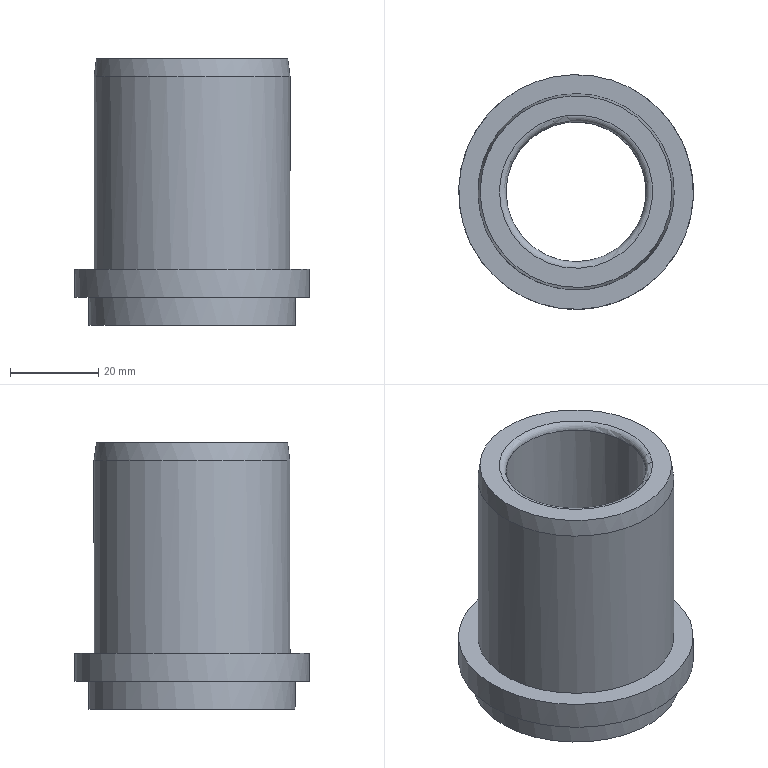Part | STEP file | 1_id1126_x_t | 1 solid | 11 faces | box 53.213 x 53.213 x 60.325 mm | volume 50805 mm3 | plane 4 | cylinder 4 | torus 2 | cone 1 | commonest cylinder face diameters 31.75 x1 44.45 x1 46.812 x1 53.213 x1
STEP:
#1=CARTESIAN_POINT('',(0.,0.,0.));
#2=DIRECTION('',(0.,0.,1.));
#3=DIRECTION('',(1.,0.,0.));
#4=AXIS2_PLACEMENT_3D('',#1,#2,#3);
#5=CARTESIAN_POINT('',(81.739,358.363,137.735));
#6=VERTEX_POINT('',#5);
#7=CARTESIAN_POINT('',(62.925,347.5,137.735));
#8=DIRECTION('',(0.,0.,1.));
#9=DIRECTION('',(0.866,0.5,0.));
#10=AXIS2_PLACEMENT_3D('',#7,#8,#9);
#11=CIRCLE('',#10,21.725);
#12=CARTESIAN_POINT('',(45.604,337.5,137.735));
#13=DIRECTION('',(0.,0.,1.));
#14=DIRECTION('',(-0.866,-0.5,0.));
#15=AXIS2_PLACEMENT_3D('',#12,#13,#14);
#16=PLANE('',#15);
#17=CARTESIAN_POINT('',(-20.,0.));
#18=DIRECTION('',(-1.,0.));
#19=AXIS2_PLACEMENT_2D('',#17,#18);
#20=CIRCLE('',#19,21.725);
#21=(GEOMETRIC_REPRESENTATION_CONTEXT(2)PARAMETRIC_REPRESENTATION_CONTEXT()REPRESENTATION_CONTEXT('',''));
#22=DEFINITIONAL_REPRESENTATION('',(#20),#21);
#23=PCURVE('',#16,#22);
#24=CARTESIAN_POINT('',(62.925,347.5,135.735));
#25=DIRECTION('',(0.,0.,-1.));
#26=DIRECTION('',(0.866,0.5,0.));
#27=AXIS2_PLACEMENT_3D('',#24,#25,#26);
#28=CONICAL_SURFACE('',#27,21.975,0.1244);
#29=CARTESIAN_POINT('',(6.283,-2.));
#30=DIRECTION('',(-1.,0.));
#31=VECTOR('',#30,1.);
#32=LINE('',#29,#31);
#33=(GEOMETRIC_REPRESENTATION_CONTEXT(2)PARAMETRIC_REPRESENTATION_CONTEXT()REPRESENTATION_CONTEXT('',''));
#34=DEFINITIONAL_REPRESENTATION('',(#32),#33);
#35=PCURVE('',#28,#34);
#36=SURFACE_CURVE('',#11,(#23,#35),.PCURVE_S1.);
#37=EDGE_CURVE('',#6,#6,#36,.T.);
#38=ORIENTED_EDGE('',*,*,#37,.T.);
#39=EDGE_LOOP('',(#38));
#40=FACE_BOUND('',#39,.T.);
#41=CARTESIAN_POINT('',(77.972,356.188,137.735));
#42=VERTEX_POINT('',#41);
#43=CARTESIAN_POINT('',(54.237,362.547,137.735));
#44=VERTEX_POINT('',#43);
#45=CARTESIAN_POINT('',(62.925,347.5,137.735));
#46=DIRECTION('',(0.,0.,-1.));
#47=DIRECTION('',(0.866,0.5,0.));
#48=AXIS2_PLACEMENT_3D('',#45,#46,#47);
#49=CIRCLE('',#48,17.375);
#50=CARTESIAN_POINT('',(-37.375,0.));
#51=CARTESIAN_POINT('',(-37.375,30.094));
#52=CARTESIAN_POINT('',(-11.312,15.047));
#53=CARTESIAN_POINT('',(14.75,0.));
#54=CARTESIAN_POINT('',(-11.312,-15.047));
#55=CARTESIAN_POINT('',(-37.375,-30.094));
#56=CARTESIAN_POINT('',(-37.375,0.));
#57=(BOUNDED_CURVE()B_SPLINE_CURVE(2,(#50,#51,#52,#53,#54,#55,#56),.UNSPECIFIED.,.T.,.F.)B_SPLINE_CURVE_WITH_KNOTS((1,2,2,2,2,1),(-2.094,0.,2.094,4.189,6.283,8.378),.UNSPECIFIED.)CURVE()GEOMETRIC_REPRESENTATION_ITEM()RATIONAL_B_SPLINE_CURVE((1.,0.5,1.,0.5,1.,0.5,1.))REPRESENTATION_ITEM(''));
#58=(GEOMETRIC_REPRESENTATION_CONTEXT(2)PARAMETRIC_REPRESENTATION_CONTEXT()REPRESENTATION_CONTEXT('',''));
#59=DEFINITIONAL_REPRESENTATION('',(#57),#58);
#60=PCURVE('',#16,#59);
#61=CARTESIAN_POINT('',(62.925,347.5,136.235));
#62=DIRECTION('',(0.,0.,1.));
#63=DIRECTION('',(-0.866,-0.5,0.));
#64=AXIS2_PLACEMENT_3D('',#61,#62,#63);
#65=TOROIDAL_SURFACE('',#64,17.375,1.5);
#66=CARTESIAN_POINT('',(9.425,7.854));
#67=DIRECTION('',(-1.,0.));
#68=VECTOR('',#67,1.);
#69=LINE('',#66,#68);
#70=(GEOMETRIC_REPRESENTATION_CONTEXT(2)PARAMETRIC_REPRESENTATION_CONTEXT()REPRESENTATION_CONTEXT('',''));
#71=DEFINITIONAL_REPRESENTATION('',(#69),#70);
#72=PCURVE('',#65,#71);
#73=SURFACE_CURVE('',#49,(#60,#72),.PCURVE_S1.);
#74=EDGE_CURVE('',#42,#44,#73,.T.);
#75=ORIENTED_EDGE('',*,*,#74,.T.);
#76=CARTESIAN_POINT('',(62.925,347.5,137.735));
#77=DIRECTION('',(0.,0.,-1.));
#78=DIRECTION('',(0.866,0.5,0.));
#79=AXIS2_PLACEMENT_3D('',#76,#77,#78);
#80=CIRCLE('',#79,17.375);
#81=CARTESIAN_POINT('',(-37.375,0.));
#82=CARTESIAN_POINT('',(-37.375,30.094));
#83=CARTESIAN_POINT('',(-11.312,15.047));
#84=CARTESIAN_POINT('',(14.75,0.));
#85=CARTESIAN_POINT('',(-11.312,-15.047));
#86=CARTESIAN_POINT('',(-37.375,-30.094));
#87=CARTESIAN_POINT('',(-37.375,0.));
#88=(BOUNDED_CURVE()B_SPLINE_CURVE(2,(#81,#82,#83,#84,#85,#86,#87),.UNSPECIFIED.,.T.,.F.)B_SPLINE_CURVE_WITH_KNOTS((1,2,2,2,2,1),(-2.094,0.,2.094,4.189,6.283,8.378),.UNSPECIFIED.)CURVE()GEOMETRIC_REPRESENTATION_ITEM()RATIONAL_B_SPLINE_CURVE((1.,0.5,1.,0.5,1.,0.5,1.))REPRESENTATION_ITEM(''));
#89=(GEOMETRIC_REPRESENTATION_CONTEXT(2)PARAMETRIC_REPRESENTATION_CONTEXT()REPRESENTATION_CONTEXT('',''));
#90=DEFINITIONAL_REPRESENTATION('',(#88),#89);
#91=PCURVE('',#16,#90);
#92=CARTESIAN_POINT('',(15.708,7.854));
#93=DIRECTION('',(-1.,0.));
#94=VECTOR('',#93,1.);
#95=LINE('',#92,#94);
#96=(GEOMETRIC_REPRESENTATION_CONTEXT(2)PARAMETRIC_REPRESENTATION_CONTEXT()REPRESENTATION_CONTEXT('',''));
#97=DEFINITIONAL_REPRESENTATION('',(#95),#96);
#98=PCURVE('',#65,#97);
#99=SURFACE_CURVE('',#80,(#91,#98),.PCURVE_S1.);
#100=EDGE_CURVE('',#44,#42,#99,.T.);
#101=ORIENTED_EDGE('',*,*,#100,.T.);
#102=EDGE_LOOP('',(#75,#101));
#103=FACE_BOUND('',#102,.T.);
#104=ADVANCED_FACE('',(#40,#103),#16,.T.);
#105=CARTESIAN_POINT('',(82.172,358.613,133.735));
#106=VERTEX_POINT('',#105);
#107=CARTESIAN_POINT('',(51.812,366.747,133.735));
#108=VERTEX_POINT('',#107);
#109=CARTESIAN_POINT('',(62.925,347.5,133.735));
#110=DIRECTION('',(0.,0.,1.));
#111=DIRECTION('',(0.866,0.5,0.));
#112=AXIS2_PLACEMENT_3D('',#109,#110,#111);
#113=CIRCLE('',#112,22.225);
#114=CARTESIAN_POINT('',(6.283,2.));
#115=DIRECTION('',(-1.,0.));
#116=VECTOR('',#115,1.);
#117=LINE('',#114,#116);
#118=(GEOMETRIC_REPRESENTATION_CONTEXT(2)PARAMETRIC_REPRESENTATION_CONTEXT()REPRESENTATION_CONTEXT('',''));
#119=DEFINITIONAL_REPRESENTATION('',(#117),#118);
#120=PCURVE('',#28,#119);
#121=CARTESIAN_POINT('',(62.925,347.5,91.735));
#122=DIRECTION('',(0.,0.,1.));
#123=DIRECTION('',(-0.5,0.866,0.));
#124=AXIS2_PLACEMENT_3D('',#121,#122,#123);
#125=CYLINDRICAL_SURFACE('',#124,22.225);
#126=CARTESIAN_POINT('',(4.712,42.));
#127=DIRECTION('',(1.,0.));
#128=VECTOR('',#127,1.);
#129=LINE('',#126,#128);
#130=(GEOMETRIC_REPRESENTATION_CONTEXT(2)PARAMETRIC_REPRESENTATION_CONTEXT()REPRESENTATION_CONTEXT('',''));
#131=DEFINITIONAL_REPRESENTATION('',(#129),#130);
#132=PCURVE('',#125,#131);
#133=SURFACE_CURVE('',#113,(#120,#132),.PCURVE_S1.);
#134=EDGE_CURVE('',#106,#108,#133,.T.);
#135=ORIENTED_EDGE('',*,*,#134,.T.);
#136=CARTESIAN_POINT('',(62.925,347.5,133.735));
#137=DIRECTION('',(0.,0.,1.));
#138=DIRECTION('',(0.866,0.5,0.));
#139=AXIS2_PLACEMENT_3D('',#136,#137,#138);
#140=CIRCLE('',#139,22.225);
#141=CARTESIAN_POINT('',(6.283,2.));
#142=DIRECTION('',(-1.,0.));
#143=VECTOR('',#142,1.);
#144=LINE('',#141,#143);
#145=(GEOMETRIC_REPRESENTATION_CONTEXT(2)PARAMETRIC_REPRESENTATION_CONTEXT()REPRESENTATION_CONTEXT('',''));
#146=DEFINITIONAL_REPRESENTATION('',(#144),#145);
#147=PCURVE('',#28,#146);
#148=CARTESIAN_POINT('',(-1.571,42.));
#149=DIRECTION('',(1.,0.));
#150=VECTOR('',#149,1.);
#151=LINE('',#148,#150);
#152=(GEOMETRIC_REPRESENTATION_CONTEXT(2)PARAMETRIC_REPRESENTATION_CONTEXT()REPRESENTATION_CONTEXT('',''));
#153=DEFINITIONAL_REPRESENTATION('',(#151),#152);
#154=PCURVE('',#125,#153);
#155=SURFACE_CURVE('',#140,(#147,#154),.PCURVE_S1.);
#156=EDGE_CURVE('',#108,#106,#155,.T.);
#157=ORIENTED_EDGE('',*,*,#156,.T.);
#158=CARTESIAN_POINT('',(81.739,358.363,137.735));
#159=CARTESIAN_POINT('',(82.172,358.612,133.735));
#160=B_SPLINE_CURVE_WITH_KNOTS('',1,(#158,#159),.UNSPECIFIED.,.F.,.F.,(2,2),(-2.016,2.016),.PIECEWISE_BEZIER_KNOTS.);
#161=CARTESIAN_POINT('',(0.,0.));
#162=DIRECTION('',(0.,1.));
#163=VECTOR('',#162,1.);
#164=LINE('',#161,#163);
#165=(GEOMETRIC_REPRESENTATION_CONTEXT(2)PARAMETRIC_REPRESENTATION_CONTEXT()REPRESENTATION_CONTEXT('',''));
#166=DEFINITIONAL_REPRESENTATION('',(#164),#165);
#167=PCURVE('',#28,#166);
#168=CARTESIAN_POINT('',(6.283,0.));
#169=DIRECTION('',(0.,1.));
#170=VECTOR('',#169,1.);
#171=LINE('',#168,#170);
#172=(GEOMETRIC_REPRESENTATION_CONTEXT(2)PARAMETRIC_REPRESENTATION_CONTEXT()REPRESENTATION_CONTEXT('',''));
#173=DEFINITIONAL_REPRESENTATION('',(#171),#172);
#174=PCURVE('',#28,#173);
#175=SEAM_CURVE('',#160,(#167,#174),.PCURVE_S1.);
#176=EDGE_CURVE('',#6,#106,#175,.T.);
#177=ORIENTED_EDGE('',*,*,#176,.F.);
#178=ORIENTED_EDGE('',*,*,#37,.F.);
#179=ORIENTED_EDGE('',*,*,#176,.T.);
#180=EDGE_LOOP('',(#135,#157,#177,#178,#179));
#181=FACE_BOUND('',#180,.T.);
#182=ADVANCED_FACE('',(#181),#28,.T.);
#183=ORIENTED_EDGE('',*,*,#156,.F.);
#184=CARTESIAN_POINT('',(51.812,366.747,90.11));
#185=VERTEX_POINT('',#184);
#186=CARTESIAN_POINT('',(51.812,366.747,90.11));
#187=CARTESIAN_POINT('',(51.812,366.747,133.735));
#188=B_SPLINE_CURVE_WITH_KNOTS('',1,(#186,#187),.UNSPECIFIED.,.F.,.F.,(2,2),(-1.625,42.),.PIECEWISE_BEZIER_KNOTS.);
#189=CARTESIAN_POINT('',(0.,0.));
#190=DIRECTION('',(0.,1.));
#191=VECTOR('',#190,1.);
#192=LINE('',#189,#191);
#193=(GEOMETRIC_REPRESENTATION_CONTEXT(2)PARAMETRIC_REPRESENTATION_CONTEXT()REPRESENTATION_CONTEXT('',''));
#194=DEFINITIONAL_REPRESENTATION('',(#192),#193);
#195=PCURVE('',#125,#194);
#196=CARTESIAN_POINT('',(6.283,0.));
#197=DIRECTION('',(0.,1.));
#198=VECTOR('',#197,1.);
#199=LINE('',#196,#198);
#200=(GEOMETRIC_REPRESENTATION_CONTEXT(2)PARAMETRIC_REPRESENTATION_CONTEXT()REPRESENTATION_CONTEXT('',''));
#201=DEFINITIONAL_REPRESENTATION('',(#199),#200);
#202=PCURVE('',#125,#201);
#203=SEAM_CURVE('',#188,(#195,#202),.PCURVE_S1.);
#204=EDGE_CURVE('',#185,#108,#203,.T.);
#205=ORIENTED_EDGE('',*,*,#204,.F.);
#206=CARTESIAN_POINT('',(62.925,347.5,90.11));
#207=DIRECTION('',(0.,0.,-1.));
#208=DIRECTION('',(-0.5,0.866,0.));
#209=AXIS2_PLACEMENT_3D('',#206,#207,#208);
#210=CIRCLE('',#209,22.225);
#211=CARTESIAN_POINT('',(6.283,-1.625));
#212=DIRECTION('',(-1.,0.));
#213=VECTOR('',#212,1.);
#214=LINE('',#211,#213);
#215=(GEOMETRIC_REPRESENTATION_CONTEXT(2)PARAMETRIC_REPRESENTATION_CONTEXT()REPRESENTATION_CONTEXT('',''));
#216=DEFINITIONAL_REPRESENTATION('',(#214),#215);
#217=PCURVE('',#125,#216);
#218=CARTESIAN_POINT('',(41.274,335.,90.11));
#219=DIRECTION('',(0.,0.,1.));
#220=DIRECTION('',(-0.866,-0.5,0.));
#221=AXIS2_PLACEMENT_3D('',#218,#219,#220);
#222=PLANE('',#221);
#223=CARTESIAN_POINT('',(-25.,-22.225));
#224=CARTESIAN_POINT('',(-63.495,-22.225));
#225=CARTESIAN_POINT('',(-44.247,11.113));
#226=CARTESIAN_POINT('',(-25.,44.45));
#227=CARTESIAN_POINT('',(-5.753,11.113));
#228=CARTESIAN_POINT('',(13.495,-22.225));
#229=CARTESIAN_POINT('',(-25.,-22.225));
#230=(BOUNDED_CURVE()B_SPLINE_CURVE(2,(#223,#224,#225,#226,#227,#228,#229),.UNSPECIFIED.,.T.,.F.)B_SPLINE_CURVE_WITH_KNOTS((1,2,2,2,2,1),(-2.094,0.,2.094,4.189,6.283,8.378),.UNSPECIFIED.)CURVE()GEOMETRIC_REPRESENTATION_ITEM()RATIONAL_B_SPLINE_CURVE((1.,0.5,1.,0.5,1.,0.5,1.))REPRESENTATION_ITEM(''));
#231=(GEOMETRIC_REPRESENTATION_CONTEXT(2)PARAMETRIC_REPRESENTATION_CONTEXT()REPRESENTATION_CONTEXT('',''));
#232=DEFINITIONAL_REPRESENTATION('',(#230),#231);
#233=PCURVE('',#222,#232);
#234=SURFACE_CURVE('',#210,(#217,#233),.PCURVE_S1.);
#235=EDGE_CURVE('',#185,#185,#234,.T.);
#236=ORIENTED_EDGE('',*,*,#235,.F.);
#237=ORIENTED_EDGE('',*,*,#204,.T.);
#238=ORIENTED_EDGE('',*,*,#134,.F.);
#239=EDGE_LOOP('',(#183,#205,#236,#237,#238));
#240=FACE_BOUND('',#239,.T.);
#241=ADVANCED_FACE('',(#240),#125,.T.);
#242=CARTESIAN_POINT('',(76.228,324.458,90.11));
#243=VERTEX_POINT('',#242);
#244=CARTESIAN_POINT('',(49.622,370.542,90.11));
#245=VERTEX_POINT('',#244);
#246=CARTESIAN_POINT('',(62.925,347.5,90.11));
#247=DIRECTION('',(0.,0.,1.));
#248=DIRECTION('',(0.5,-0.866,0.));
#249=AXIS2_PLACEMENT_3D('',#246,#247,#248);
#250=CIRCLE('',#249,26.606);
#251=CARTESIAN_POINT('',(-25.,0.));
#252=DIRECTION('',(0.,1.));
#253=AXIS2_PLACEMENT_2D('',#251,#252);
#254=CIRCLE('',#253,26.606);
#255=(GEOMETRIC_REPRESENTATION_CONTEXT(2)PARAMETRIC_REPRESENTATION_CONTEXT()REPRESENTATION_CONTEXT('',''));
#256=DEFINITIONAL_REPRESENTATION('',(#254),#255);
#257=PCURVE('',#222,#256);
#258=CARTESIAN_POINT('',(62.925,347.5,84.11));
#259=DIRECTION('',(0.,0.,1.));
#260=DIRECTION('',(-0.5,0.866,0.));
#261=AXIS2_PLACEMENT_3D('',#258,#259,#260);
#262=CYLINDRICAL_SURFACE('',#261,26.606);
#263=CARTESIAN_POINT('',(3.142,6.));
#264=DIRECTION('',(1.,0.));
#265=VECTOR('',#264,1.);
#266=LINE('',#263,#265);
#267=(GEOMETRIC_REPRESENTATION_CONTEXT(2)PARAMETRIC_REPRESENTATION_CONTEXT()REPRESENTATION_CONTEXT('',''));
#268=DEFINITIONAL_REPRESENTATION('',(#266),#267);
#269=PCURVE('',#262,#268);
#270=SURFACE_CURVE('',#250,(#257,#269),.PCURVE_S1.);
#271=EDGE_CURVE('',#243,#245,#270,.T.);
#272=ORIENTED_EDGE('',*,*,#271,.T.);
#273=CARTESIAN_POINT('',(62.925,347.5,90.11));
#274=DIRECTION('',(0.,0.,1.));
#275=DIRECTION('',(0.5,-0.866,0.));
#276=AXIS2_PLACEMENT_3D('',#273,#274,#275);
#277=CIRCLE('',#276,26.606);
#278=CARTESIAN_POINT('',(-25.,0.));
#279=DIRECTION('',(0.,1.));
#280=AXIS2_PLACEMENT_2D('',#278,#279);
#281=CIRCLE('',#280,26.606);
#282=(GEOMETRIC_REPRESENTATION_CONTEXT(2)PARAMETRIC_REPRESENTATION_CONTEXT()REPRESENTATION_CONTEXT('',''));
#283=DEFINITIONAL_REPRESENTATION('',(#281),#282);
#284=PCURVE('',#222,#283);
#285=CARTESIAN_POINT('',(-3.142,6.));
#286=DIRECTION('',(1.,0.));
#287=VECTOR('',#286,1.);
#288=LINE('',#285,#287);
#289=(GEOMETRIC_REPRESENTATION_CONTEXT(2)PARAMETRIC_REPRESENTATION_CONTEXT()REPRESENTATION_CONTEXT('',''));
#290=DEFINITIONAL_REPRESENTATION('',(#288),#289);
#291=PCURVE('',#262,#290);
#292=SURFACE_CURVE('',#277,(#284,#291),.PCURVE_S1.);
#293=EDGE_CURVE('',#245,#243,#292,.T.);
#294=ORIENTED_EDGE('',*,*,#293,.T.);
#295=EDGE_LOOP('',(#272,#294));
#296=FACE_BOUND('',#295,.T.);
#297=ORIENTED_EDGE('',*,*,#235,.T.);
#298=EDGE_LOOP('',(#297));
#299=FACE_BOUND('',#298,.T.);
#300=ADVANCED_FACE('',(#296,#299),#222,.T.);
#301=ORIENTED_EDGE('',*,*,#293,.F.);
#302=CARTESIAN_POINT('',(49.622,370.542,83.76));
#303=VERTEX_POINT('',#302);
#304=CARTESIAN_POINT('',(49.622,370.542,83.76));
#305=CARTESIAN_POINT('',(49.622,370.542,90.11));
#306=B_SPLINE_CURVE_WITH_KNOTS('',1,(#304,#305),.UNSPECIFIED.,.F.,.F.,(2,2),(-0.35,6.),.PIECEWISE_BEZIER_KNOTS.);
#307=CARTESIAN_POINT('',(0.,0.));
#308=DIRECTION('',(0.,1.));
#309=VECTOR('',#308,1.);
#310=LINE('',#307,#309);
#311=(GEOMETRIC_REPRESENTATION_CONTEXT(2)PARAMETRIC_REPRESENTATION_CONTEXT()REPRESENTATION_CONTEXT('',''));
#312=DEFINITIONAL_REPRESENTATION('',(#310),#311);
#313=PCURVE('',#262,#312);
#314=CARTESIAN_POINT('',(6.283,0.));
#315=DIRECTION('',(0.,1.));
#316=VECTOR('',#315,1.);
#317=LINE('',#314,#316);
#318=(GEOMETRIC_REPRESENTATION_CONTEXT(2)PARAMETRIC_REPRESENTATION_CONTEXT()REPRESENTATION_CONTEXT('',''));
#319=DEFINITIONAL_REPRESENTATION('',(#317),#318);
#320=PCURVE('',#262,#319);
#321=SEAM_CURVE('',#306,(#313,#320),.PCURVE_S1.);
#322=EDGE_CURVE('',#303,#245,#321,.T.);
#323=ORIENTED_EDGE('',*,*,#322,.F.);
#324=CARTESIAN_POINT('',(62.925,347.5,83.76));
#325=DIRECTION('',(0.,0.,-1.));
#326=DIRECTION('',(-0.5,0.866,0.));
#327=AXIS2_PLACEMENT_3D('',#324,#325,#326);
#328=CIRCLE('',#327,26.606);
#329=CARTESIAN_POINT('',(6.283,-0.35));
#330=DIRECTION('',(-1.,0.));
#331=VECTOR('',#330,1.);
#332=LINE('',#329,#331);
#333=(GEOMETRIC_REPRESENTATION_CONTEXT(2)PARAMETRIC_REPRESENTATION_CONTEXT()REPRESENTATION_CONTEXT('',''));
#334=DEFINITIONAL_REPRESENTATION('',(#332),#333);
#335=PCURVE('',#262,#334);
#336=CARTESIAN_POINT('',(45.604,337.5,83.76));
#337=DIRECTION('',(0.,0.,-1.));
#338=DIRECTION('',(-0.5,0.866,0.));
#339=AXIS2_PLACEMENT_3D('',#336,#337,#338);
#340=PLANE('',#339);
#341=CARTESIAN_POINT('',(0.,20.));
#342=DIRECTION('',(1.,0.));
#343=AXIS2_PLACEMENT_2D('',#341,#342);
#344=CIRCLE('',#343,26.606);
#345=(GEOMETRIC_REPRESENTATION_CONTEXT(2)PARAMETRIC_REPRESENTATION_CONTEXT()REPRESENTATION_CONTEXT('',''));
#346=DEFINITIONAL_REPRESENTATION('',(#344),#345);
#347=PCURVE('',#340,#346);
#348=SURFACE_CURVE('',#328,(#335,#347),.PCURVE_S1.);
#349=EDGE_CURVE('',#303,#303,#348,.T.);
#350=ORIENTED_EDGE('',*,*,#349,.F.);
#351=ORIENTED_EDGE('',*,*,#322,.T.);
#352=ORIENTED_EDGE('',*,*,#271,.F.);
#353=EDGE_LOOP('',(#301,#323,#350,#351,#352));
#354=FACE_BOUND('',#353,.T.);
#355=ADVANCED_FACE('',(#354),#262,.T.);
#356=ORIENTED_EDGE('',*,*,#349,.T.);
#357=EDGE_LOOP('',(#356));
#358=FACE_BOUND('',#357,.T.);
#359=CARTESIAN_POINT('',(74.628,327.23,83.76));
#360=VERTEX_POINT('',#359);
#361=CARTESIAN_POINT('',(51.222,367.77,83.76));
#362=VERTEX_POINT('',#361);
#363=CARTESIAN_POINT('',(62.925,347.5,83.76));
#364=DIRECTION('',(0.,0.,1.));
#365=DIRECTION('',(0.5,-0.866,0.));
#366=AXIS2_PLACEMENT_3D('',#363,#364,#365);
#367=CIRCLE('',#366,23.406);
#368=CARTESIAN_POINT('',(-23.406,20.));
#369=CARTESIAN_POINT('',(-23.406,60.541));
#370=CARTESIAN_POINT('',(11.703,40.27));
#371=CARTESIAN_POINT('',(46.812,20.));
#372=CARTESIAN_POINT('',(11.703,-0.2703));
#373=CARTESIAN_POINT('',(-23.406,-20.541));
#374=CARTESIAN_POINT('',(-23.406,20.));
#375=(BOUNDED_CURVE()B_SPLINE_CURVE(2,(#368,#369,#370,#371,#372,#373,#374),.UNSPECIFIED.,.T.,.F.)B_SPLINE_CURVE_WITH_KNOTS((1,2,2,2,2,1),(-2.094,0.,2.094,4.189,6.283,8.378),.UNSPECIFIED.)CURVE()GEOMETRIC_REPRESENTATION_ITEM()RATIONAL_B_SPLINE_CURVE((1.,0.5,1.,0.5,1.,0.5,1.))REPRESENTATION_ITEM(''));
#376=(GEOMETRIC_REPRESENTATION_CONTEXT(2)PARAMETRIC_REPRESENTATION_CONTEXT()REPRESENTATION_CONTEXT('',''));
#377=DEFINITIONAL_REPRESENTATION('',(#375),#376);
#378=PCURVE('',#340,#377);
#379=CARTESIAN_POINT('',(62.925,347.5,84.11));
#380=DIRECTION('',(0.,0.,1.));
#381=DIRECTION('',(-0.5,0.866,0.));
#382=AXIS2_PLACEMENT_3D('',#379,#380,#381);
#383=CYLINDRICAL_SURFACE('',#382,23.406);
#384=CARTESIAN_POINT('',(3.142,-0.35));
#385=DIRECTION('',(1.,0.));
#386=VECTOR('',#385,1.);
#387=LINE('',#384,#386);
#388=(GEOMETRIC_REPRESENTATION_CONTEXT(2)PARAMETRIC_REPRESENTATION_CONTEXT()REPRESENTATION_CONTEXT('',''));
#389=DEFINITIONAL_REPRESENTATION('',(#387),#388);
#390=PCURVE('',#383,#389);
#391=SURFACE_CURVE('',#367,(#378,#390),.PCURVE_S1.);
#392=EDGE_CURVE('',#360,#362,#391,.T.);
#393=ORIENTED_EDGE('',*,*,#392,.T.);
#394=CARTESIAN_POINT('',(62.925,347.5,83.76));
#395=DIRECTION('',(0.,0.,1.));
#396=DIRECTION('',(0.5,-0.866,0.));
#397=AXIS2_PLACEMENT_3D('',#394,#395,#396);
#398=CIRCLE('',#397,23.406);
#399=CARTESIAN_POINT('',(-23.406,20.));
#400=CARTESIAN_POINT('',(-23.406,60.541));
#401=CARTESIAN_POINT('',(11.703,40.27));
#402=CARTESIAN_POINT('',(46.812,20.));
#403=CARTESIAN_POINT('',(11.703,-0.2703));
#404=CARTESIAN_POINT('',(-23.406,-20.541));
#405=CARTESIAN_POINT('',(-23.406,20.));
#406=(BOUNDED_CURVE()B_SPLINE_CURVE(2,(#399,#400,#401,#402,#403,#404,#405),.UNSPECIFIED.,.T.,.F.)B_SPLINE_CURVE_WITH_KNOTS((1,2,2,2,2,1),(-2.094,0.,2.094,4.189,6.283,8.378),.UNSPECIFIED.)CURVE()GEOMETRIC_REPRESENTATION_ITEM()RATIONAL_B_SPLINE_CURVE((1.,0.5,1.,0.5,1.,0.5,1.))REPRESENTATION_ITEM(''));
#407=(GEOMETRIC_REPRESENTATION_CONTEXT(2)PARAMETRIC_REPRESENTATION_CONTEXT()REPRESENTATION_CONTEXT('',''));
#408=DEFINITIONAL_REPRESENTATION('',(#406),#407);
#409=PCURVE('',#340,#408);
#410=CARTESIAN_POINT('',(-3.142,-0.35));
#411=DIRECTION('',(1.,0.));
#412=VECTOR('',#411,1.);
#413=LINE('',#410,#412);
#414=(GEOMETRIC_REPRESENTATION_CONTEXT(2)PARAMETRIC_REPRESENTATION_CONTEXT()REPRESENTATION_CONTEXT('',''));
#415=DEFINITIONAL_REPRESENTATION('',(#413),#414);
#416=PCURVE('',#383,#415);
#417=SURFACE_CURVE('',#398,(#409,#416),.PCURVE_S1.);
#418=EDGE_CURVE('',#362,#360,#417,.T.);
#419=ORIENTED_EDGE('',*,*,#418,.T.);
#420=EDGE_LOOP('',(#393,#419));
#421=FACE_BOUND('',#420,.T.);
#422=ADVANCED_FACE('',(#358,#421),#340,.T.);
#423=ORIENTED_EDGE('',*,*,#418,.F.);
#424=CARTESIAN_POINT('',(51.222,367.77,77.41));
#425=VERTEX_POINT('',#424);
#426=CARTESIAN_POINT('',(51.222,367.77,77.41));
#427=CARTESIAN_POINT('',(51.222,367.77,83.76));
#428=B_SPLINE_CURVE_WITH_KNOTS('',1,(#426,#427),.UNSPECIFIED.,.F.,.F.,(2,2),(-6.7,-0.35),.PIECEWISE_BEZIER_KNOTS.);
#429=CARTESIAN_POINT('',(0.,0.));
#430=DIRECTION('',(0.,1.));
#431=VECTOR('',#430,1.);
#432=LINE('',#429,#431);
#433=(GEOMETRIC_REPRESENTATION_CONTEXT(2)PARAMETRIC_REPRESENTATION_CONTEXT()REPRESENTATION_CONTEXT('',''));
#434=DEFINITIONAL_REPRESENTATION('',(#432),#433);
#435=PCURVE('',#383,#434);
#436=CARTESIAN_POINT('',(6.283,0.));
#437=DIRECTION('',(0.,1.));
#438=VECTOR('',#437,1.);
#439=LINE('',#436,#438);
#440=(GEOMETRIC_REPRESENTATION_CONTEXT(2)PARAMETRIC_REPRESENTATION_CONTEXT()REPRESENTATION_CONTEXT('',''));
#441=DEFINITIONAL_REPRESENTATION('',(#439),#440);
#442=PCURVE('',#383,#441);
#443=SEAM_CURVE('',#428,(#435,#442),.PCURVE_S1.);
#444=EDGE_CURVE('',#425,#362,#443,.T.);
#445=ORIENTED_EDGE('',*,*,#444,.F.);
#446=CARTESIAN_POINT('',(62.925,347.5,77.41));
#447=DIRECTION('',(0.,0.,-1.));
#448=DIRECTION('',(-0.5,0.866,0.));
#449=AXIS2_PLACEMENT_3D('',#446,#447,#448);
#450=CIRCLE('',#449,23.406);
#451=CARTESIAN_POINT('',(6.283,-6.7));
#452=DIRECTION('',(-1.,0.));
#453=VECTOR('',#452,1.);
#454=LINE('',#451,#453);
#455=(GEOMETRIC_REPRESENTATION_CONTEXT(2)PARAMETRIC_REPRESENTATION_CONTEXT()REPRESENTATION_CONTEXT('',''));
#456=DEFINITIONAL_REPRESENTATION('',(#454),#455);
#457=PCURVE('',#383,#456);
#458=CARTESIAN_POINT('',(49.069,339.5,77.41));
#459=DIRECTION('',(0.,0.,-1.));
#460=DIRECTION('',(-0.5,0.866,0.));
#461=AXIS2_PLACEMENT_3D('',#458,#459,#460);
#462=PLANE('',#461);
#463=CARTESIAN_POINT('',(0.,16.));
#464=DIRECTION('',(1.,0.));
#465=AXIS2_PLACEMENT_2D('',#463,#464);
#466=CIRCLE('',#465,23.406);
#467=(GEOMETRIC_REPRESENTATION_CONTEXT(2)PARAMETRIC_REPRESENTATION_CONTEXT()REPRESENTATION_CONTEXT('',''));
#468=DEFINITIONAL_REPRESENTATION('',(#466),#467);
#469=PCURVE('',#462,#468);
#470=SURFACE_CURVE('',#450,(#457,#469),.PCURVE_S1.);
#471=EDGE_CURVE('',#425,#425,#470,.T.);
#472=ORIENTED_EDGE('',*,*,#471,.F.);
#473=ORIENTED_EDGE('',*,*,#444,.T.);
#474=ORIENTED_EDGE('',*,*,#392,.F.);
#475=EDGE_LOOP('',(#423,#445,#472,#473,#474));
#476=FACE_BOUND('',#475,.T.);
#477=ADVANCED_FACE('',(#476),#383,.T.);
#478=ORIENTED_EDGE('',*,*,#471,.T.);
#479=EDGE_LOOP('',(#478));
#480=FACE_BOUND('',#479,.T.);
#481=CARTESIAN_POINT('',(46.579,338.062,77.41));
#482=VERTEX_POINT('',#481);
#483=CARTESIAN_POINT('',(79.271,356.938,77.41));
#484=VERTEX_POINT('',#483);
#485=CARTESIAN_POINT('',(62.925,347.5,77.41));
#486=DIRECTION('',(0.,0.,1.));
#487=DIRECTION('',(-0.866,-0.5,0.));
#488=AXIS2_PLACEMENT_3D('',#485,#486,#487);
#489=CIRCLE('',#488,18.875);
#490=CARTESIAN_POINT('',(0.,-2.875));
#491=CARTESIAN_POINT('',(-32.692,-2.875));
#492=CARTESIAN_POINT('',(-16.346,25.437));
#493=CARTESIAN_POINT('',(0.,53.75));
#494=CARTESIAN_POINT('',(16.346,25.437));
#495=CARTESIAN_POINT('',(32.692,-2.875));
#496=CARTESIAN_POINT('',(0.,-2.875));
#497=(BOUNDED_CURVE()B_SPLINE_CURVE(2,(#490,#491,#492,#493,#494,#495,#496),.UNSPECIFIED.,.T.,.F.)B_SPLINE_CURVE_WITH_KNOTS((1,2,2,2,2,1),(-2.094,0.,2.094,4.189,6.283,8.378),.UNSPECIFIED.)CURVE()GEOMETRIC_REPRESENTATION_ITEM()RATIONAL_B_SPLINE_CURVE((1.,0.5,1.,0.5,1.,0.5,1.))REPRESENTATION_ITEM(''));
#498=(GEOMETRIC_REPRESENTATION_CONTEXT(2)PARAMETRIC_REPRESENTATION_CONTEXT()REPRESENTATION_CONTEXT('',''));
#499=DEFINITIONAL_REPRESENTATION('',(#497),#498);
#500=PCURVE('',#462,#499);
#501=CARTESIAN_POINT('',(62.925,347.5,80.41));
#502=DIRECTION('',(0.,0.,-1.));
#503=DIRECTION('',(0.866,0.5,0.));
#504=AXIS2_PLACEMENT_3D('',#501,#502,#503);
#505=TOROIDAL_SURFACE('',#504,18.875,3.);
#506=CARTESIAN_POINT('',(3.142,7.854));
#507=DIRECTION('',(-1.,0.));
#508=VECTOR('',#507,1.);
#509=LINE('',#506,#508);
#510=(GEOMETRIC_REPRESENTATION_CONTEXT(2)PARAMETRIC_REPRESENTATION_CONTEXT()REPRESENTATION_CONTEXT('',''));
#511=DEFINITIONAL_REPRESENTATION('',(#509),#510);
#512=PCURVE('',#505,#511);
#513=SURFACE_CURVE('',#489,(#500,#512),.PCURVE_S1.);
#514=EDGE_CURVE('',#482,#484,#513,.T.);
#515=ORIENTED_EDGE('',*,*,#514,.T.);
#516=CARTESIAN_POINT('',(62.925,347.5,77.41));
#517=DIRECTION('',(0.,0.,1.));
#518=DIRECTION('',(-0.866,-0.5,0.));
#519=AXIS2_PLACEMENT_3D('',#516,#517,#518);
#520=CIRCLE('',#519,18.875);
#521=CARTESIAN_POINT('',(0.,-2.875));
#522=CARTESIAN_POINT('',(-32.692,-2.875));
#523=CARTESIAN_POINT('',(-16.346,25.437));
#524=CARTESIAN_POINT('',(0.,53.75));
#525=CARTESIAN_POINT('',(16.346,25.437));
#526=CARTESIAN_POINT('',(32.692,-2.875));
#527=CARTESIAN_POINT('',(0.,-2.875));
#528=(BOUNDED_CURVE()B_SPLINE_CURVE(2,(#521,#522,#523,#524,#525,#526,#527),.UNSPECIFIED.,.T.,.F.)B_SPLINE_CURVE_WITH_KNOTS((1,2,2,2,2,1),(-2.094,0.,2.094,4.189,6.283,8.378),.UNSPECIFIED.)CURVE()GEOMETRIC_REPRESENTATION_ITEM()RATIONAL_B_SPLINE_CURVE((1.,0.5,1.,0.5,1.,0.5,1.))REPRESENTATION_ITEM(''));
#529=(GEOMETRIC_REPRESENTATION_CONTEXT(2)PARAMETRIC_REPRESENTATION_CONTEXT()REPRESENTATION_CONTEXT('',''));
#530=DEFINITIONAL_REPRESENTATION('',(#528),#529);
#531=PCURVE('',#462,#530);
#532=CARTESIAN_POINT('',(9.425,7.854));
#533=DIRECTION('',(-1.,0.));
#534=VECTOR('',#533,1.);
#535=LINE('',#532,#534);
#536=(GEOMETRIC_REPRESENTATION_CONTEXT(2)PARAMETRIC_REPRESENTATION_CONTEXT()REPRESENTATION_CONTEXT('',''));
#537=DEFINITIONAL_REPRESENTATION('',(#535),#536);
#538=PCURVE('',#505,#537);
#539=SURFACE_CURVE('',#520,(#531,#538),.PCURVE_S1.);
#540=EDGE_CURVE('',#484,#482,#539,.T.);
#541=ORIENTED_EDGE('',*,*,#540,.T.);
#542=EDGE_LOOP('',(#515,#541));
#543=FACE_BOUND('',#542,.T.);
#544=ADVANCED_FACE('',(#480,#543),#462,.T.);
#545=CARTESIAN_POINT('',(76.673,355.438,80.41));
#546=VERTEX_POINT('',#545);
#547=CARTESIAN_POINT('',(54.987,361.248,80.41));
#548=VERTEX_POINT('',#547);
#549=CARTESIAN_POINT('',(62.925,347.5,80.41));
#550=DIRECTION('',(0.,0.,1.));
#551=DIRECTION('',(0.866,0.5,0.));
#552=AXIS2_PLACEMENT_3D('',#549,#550,#551);
#553=CIRCLE('',#552,15.875);
#554=CARTESIAN_POINT('',(6.283,9.425));
#555=DIRECTION('',(-1.,0.));
#556=VECTOR('',#555,1.);
#557=LINE('',#554,#556);
#558=(GEOMETRIC_REPRESENTATION_CONTEXT(2)PARAMETRIC_REPRESENTATION_CONTEXT()REPRESENTATION_CONTEXT('',''));
#559=DEFINITIONAL_REPRESENTATION('',(#557),#558);
#560=PCURVE('',#505,#559);
#561=CARTESIAN_POINT('',(62.925,347.5,91.735));
#562=DIRECTION('',(0.,0.,1.));
#563=DIRECTION('',(-0.5,0.866,0.));
#564=AXIS2_PLACEMENT_3D('',#561,#562,#563);
#565=CYLINDRICAL_SURFACE('',#564,15.875);
#566=CARTESIAN_POINT('',(4.712,-11.325));
#567=DIRECTION('',(1.,0.));
#568=VECTOR('',#567,1.);
#569=LINE('',#566,#568);
#570=(GEOMETRIC_REPRESENTATION_CONTEXT(2)PARAMETRIC_REPRESENTATION_CONTEXT()REPRESENTATION_CONTEXT('',''));
#571=DEFINITIONAL_REPRESENTATION('',(#569),#570);
#572=PCURVE('',#565,#571);
#573=SURFACE_CURVE('',#553,(#560,#572),.PCURVE_S1.);
#574=EDGE_CURVE('',#546,#548,#573,.T.);
#575=ORIENTED_EDGE('',*,*,#574,.T.);
#576=CARTESIAN_POINT('',(62.925,347.5,80.41));
#577=DIRECTION('',(0.,0.,1.));
#578=DIRECTION('',(0.866,0.5,0.));
#579=AXIS2_PLACEMENT_3D('',#576,#577,#578);
#580=CIRCLE('',#579,15.875);
#581=CARTESIAN_POINT('',(6.283,9.425));
#582=DIRECTION('',(-1.,0.));
#583=VECTOR('',#582,1.);
#584=LINE('',#581,#583);
#585=(GEOMETRIC_REPRESENTATION_CONTEXT(2)PARAMETRIC_REPRESENTATION_CONTEXT()REPRESENTATION_CONTEXT('',''));
#586=DEFINITIONAL_REPRESENTATION('',(#584),#585);
#587=PCURVE('',#505,#586);
#588=CARTESIAN_POINT('',(-1.571,-11.325));
#589=DIRECTION('',(1.,0.));
#590=VECTOR('',#589,1.);
#591=LINE('',#588,#590);
#592=(GEOMETRIC_REPRESENTATION_CONTEXT(2)PARAMETRIC_REPRESENTATION_CONTEXT()REPRESENTATION_CONTEXT('',''));
#593=DEFINITIONAL_REPRESENTATION('',(#591),#592);
#594=PCURVE('',#565,#593);
#595=SURFACE_CURVE('',#580,(#587,#594),.PCURVE_S1.);
#596=EDGE_CURVE('',#548,#546,#595,.T.);
#597=ORIENTED_EDGE('',*,*,#596,.T.);
#598=CARTESIAN_POINT('',(79.271,356.938,77.41));
#599=CARTESIAN_POINT('',(78.577,356.536,77.41));
#600=CARTESIAN_POINT('',(77.9,356.146,77.665));
#601=CARTESIAN_POINT('',(77.318,355.81,78.154));
#602=CARTESIAN_POINT('',(76.894,355.565,78.827));
#603=CARTESIAN_POINT('',(76.673,355.438,79.608));
#604=CARTESIAN_POINT('',(76.673,355.438,80.41));
#605=(BOUNDED_CURVE()B_SPLINE_CURVE(6,(#598,#599,#600,#601,#602,#603,#604),.UNSPECIFIED.,.F.,.F.)B_SPLINE_CURVE_WITH_KNOTS((7,7),(1.571,3.142),.PIECEWISE_BEZIER_KNOTS.)CURVE()GEOMETRIC_REPRESENTATION_ITEM()RATIONAL_B_SPLINE_CURVE((1.031,1.01,0.9979,0.994,0.9979,1.01,1.031))REPRESENTATION_ITEM(''));
#606=CARTESIAN_POINT('',(0.,6.283));
#607=DIRECTION('',(0.,1.));
#608=VECTOR('',#607,1.);
#609=LINE('',#606,#608);
#610=(GEOMETRIC_REPRESENTATION_CONTEXT(2)PARAMETRIC_REPRESENTATION_CONTEXT()REPRESENTATION_CONTEXT('',''));
#611=DEFINITIONAL_REPRESENTATION('',(#609),#610);
#612=PCURVE('',#505,#611);
#613=CARTESIAN_POINT('',(6.283,6.283));
#614=DIRECTION('',(0.,1.));
#615=VECTOR('',#614,1.);
#616=LINE('',#613,#615);
#617=(GEOMETRIC_REPRESENTATION_CONTEXT(2)PARAMETRIC_REPRESENTATION_CONTEXT()REPRESENTATION_CONTEXT('',''));
#618=DEFINITIONAL_REPRESENTATION('',(#616),#617);
#619=PCURVE('',#505,#618);
#620=SEAM_CURVE('',#605,(#612,#619),.PCURVE_S1.);
#621=EDGE_CURVE('',#484,#546,#620,.T.);
#622=ORIENTED_EDGE('',*,*,#621,.F.);
#623=ORIENTED_EDGE('',*,*,#514,.F.);
#624=ORIENTED_EDGE('',*,*,#540,.F.);
#625=ORIENTED_EDGE('',*,*,#621,.T.);
#626=EDGE_LOOP('',(#575,#597,#622,#623,#624,#625));
#627=FACE_BOUND('',#626,.T.);
#628=ADVANCED_FACE('',(#627),#505,.T.);
#629=CARTESIAN_POINT('',(54.987,361.248,136.235));
#630=VERTEX_POINT('',#629);
#631=CARTESIAN_POINT('',(62.925,347.5,136.235));
#632=DIRECTION('',(0.,0.,-1.));
#633=DIRECTION('',(-0.5,0.866,0.));
#634=AXIS2_PLACEMENT_3D('',#631,#632,#633);
#635=CIRCLE('',#634,15.875);
#636=CARTESIAN_POINT('',(6.283,44.5));
#637=DIRECTION('',(-1.,0.));
#638=VECTOR('',#637,1.);
#639=LINE('',#636,#638);
#640=(GEOMETRIC_REPRESENTATION_CONTEXT(2)PARAMETRIC_REPRESENTATION_CONTEXT()REPRESENTATION_CONTEXT('',''));
#641=DEFINITIONAL_REPRESENTATION('',(#639),#640);
#642=PCURVE('',#565,#641);
#643=CARTESIAN_POINT('',(10.996,9.425));
#644=DIRECTION('',(-1.,0.));
#645=VECTOR('',#644,1.);
#646=LINE('',#643,#645);
#647=(GEOMETRIC_REPRESENTATION_CONTEXT(2)PARAMETRIC_REPRESENTATION_CONTEXT()REPRESENTATION_CONTEXT('',''));
#648=DEFINITIONAL_REPRESENTATION('',(#646),#647);
#649=PCURVE('',#65,#648);
#650=SURFACE_CURVE('',#635,(#642,#649),.PCURVE_S1.);
#651=EDGE_CURVE('',#630,#630,#650,.T.);
#652=ORIENTED_EDGE('',*,*,#651,.T.);
#653=CARTESIAN_POINT('',(54.987,361.248,80.41));
#654=CARTESIAN_POINT('',(54.987,361.248,136.235));
#655=B_SPLINE_CURVE_WITH_KNOTS('',1,(#653,#654),.UNSPECIFIED.,.F.,.F.,(2,2),(-11.325,44.5),.PIECEWISE_BEZIER_KNOTS.);
#656=CARTESIAN_POINT('',(0.,0.));
#657=DIRECTION('',(0.,1.));
#658=VECTOR('',#657,1.);
#659=LINE('',#656,#658);
#660=(GEOMETRIC_REPRESENTATION_CONTEXT(2)PARAMETRIC_REPRESENTATION_CONTEXT()REPRESENTATION_CONTEXT('',''));
#661=DEFINITIONAL_REPRESENTATION('',(#659),#660);
#662=PCURVE('',#565,#661);
#663=CARTESIAN_POINT('',(6.283,0.));
#664=DIRECTION('',(0.,1.));
#665=VECTOR('',#664,1.);
#666=LINE('',#663,#665);
#667=(GEOMETRIC_REPRESENTATION_CONTEXT(2)PARAMETRIC_REPRESENTATION_CONTEXT()REPRESENTATION_CONTEXT('',''));
#668=DEFINITIONAL_REPRESENTATION('',(#666),#667);
#669=PCURVE('',#565,#668);
#670=SEAM_CURVE('',#655,(#662,#669),.PCURVE_S1.);
#671=EDGE_CURVE('',#548,#630,#670,.T.);
#672=ORIENTED_EDGE('',*,*,#671,.F.);
#673=ORIENTED_EDGE('',*,*,#596,.T.);
#674=ORIENTED_EDGE('',*,*,#574,.T.);
#675=ORIENTED_EDGE('',*,*,#671,.T.);
#676=EDGE_LOOP('',(#652,#672,#673,#674,#675));
#677=FACE_BOUND('',#676,.F.);
#678=ADVANCED_FACE('',(#677),#565,.F.);
#679=ORIENTED_EDGE('',*,*,#651,.T.);
#680=CARTESIAN_POINT('',(54.237,362.547,137.735));
#681=CARTESIAN_POINT('',(54.438,362.2,137.735));
#682=CARTESIAN_POINT('',(54.633,361.862,137.607));
#683=CARTESIAN_POINT('',(54.801,361.57,137.363));
#684=CARTESIAN_POINT('',(54.924,361.359,137.027));
#685=CARTESIAN_POINT('',(54.987,361.248,136.636));
#686=CARTESIAN_POINT('',(54.987,361.248,136.235));
#687=(BOUNDED_CURVE()B_SPLINE_CURVE(6,(#680,#681,#682,#683,#684,#685,#686),.UNSPECIFIED.,.F.,.F.)B_SPLINE_CURVE_WITH_KNOTS((7,7),(1.571,3.142),.PIECEWISE_BEZIER_KNOTS.)CURVE()GEOMETRIC_REPRESENTATION_ITEM()RATIONAL_B_SPLINE_CURVE((1.031,1.01,0.9979,0.994,0.9979,1.01,1.031))REPRESENTATION_ITEM(''));
#688=CARTESIAN_POINT('',(4.712,6.283));
#689=DIRECTION('',(0.,1.));
#690=VECTOR('',#689,1.);
#691=LINE('',#688,#690);
#692=(GEOMETRIC_REPRESENTATION_CONTEXT(2)PARAMETRIC_REPRESENTATION_CONTEXT()REPRESENTATION_CONTEXT('',''));
#693=DEFINITIONAL_REPRESENTATION('',(#691),#692);
#694=PCURVE('',#65,#693);
#695=CARTESIAN_POINT('',(10.996,6.283));
#696=DIRECTION('',(0.,1.));
#697=VECTOR('',#696,1.);
#698=LINE('',#695,#697);
#699=(GEOMETRIC_REPRESENTATION_CONTEXT(2)PARAMETRIC_REPRESENTATION_CONTEXT()REPRESENTATION_CONTEXT('',''));
#700=DEFINITIONAL_REPRESENTATION('',(#698),#699);
#701=PCURVE('',#65,#700);
#702=SEAM_CURVE('',#687,(#694,#701),.PCURVE_S1.);
#703=EDGE_CURVE('',#44,#630,#702,.T.);
#704=ORIENTED_EDGE('',*,*,#703,.F.);
#705=ORIENTED_EDGE('',*,*,#74,.F.);
#706=ORIENTED_EDGE('',*,*,#100,.F.);
#707=ORIENTED_EDGE('',*,*,#703,.T.);
#708=EDGE_LOOP('',(#679,#704,#705,#706,#707));
#709=FACE_BOUND('',#708,.T.);
#710=ADVANCED_FACE('',(#709),#65,.T.);
#711=CLOSED_SHELL('',(#104,#182,#241,#300,#355,#422,#477,#544,#628,#678,#710));
#712=MANIFOLD_SOLID_BREP('',#711);
#713=(LENGTH_UNIT()NAMED_UNIT(*)SI_UNIT(.MILLI.,.METRE.));
#714=UNCERTAINTY_MEASURE_WITH_UNIT(LENGTH_MEASURE(0.000005),#713,'','');
#715=(NAMED_UNIT(*)PLANE_ANGLE_UNIT()SI_UNIT($,.RADIAN.));
#716=(NAMED_UNIT(*)SI_UNIT($,.STERADIAN.)SOLID_ANGLE_UNIT());
#717=(GEOMETRIC_REPRESENTATION_CONTEXT(3)GLOBAL_UNCERTAINTY_ASSIGNED_CONTEXT((#714))GLOBAL_UNIT_ASSIGNED_CONTEXT((#713,#715,#716))REPRESENTATION_CONTEXT('',''));
#718=ADVANCED_BREP_SHAPE_REPRESENTATION('',(#4,#712),#717);